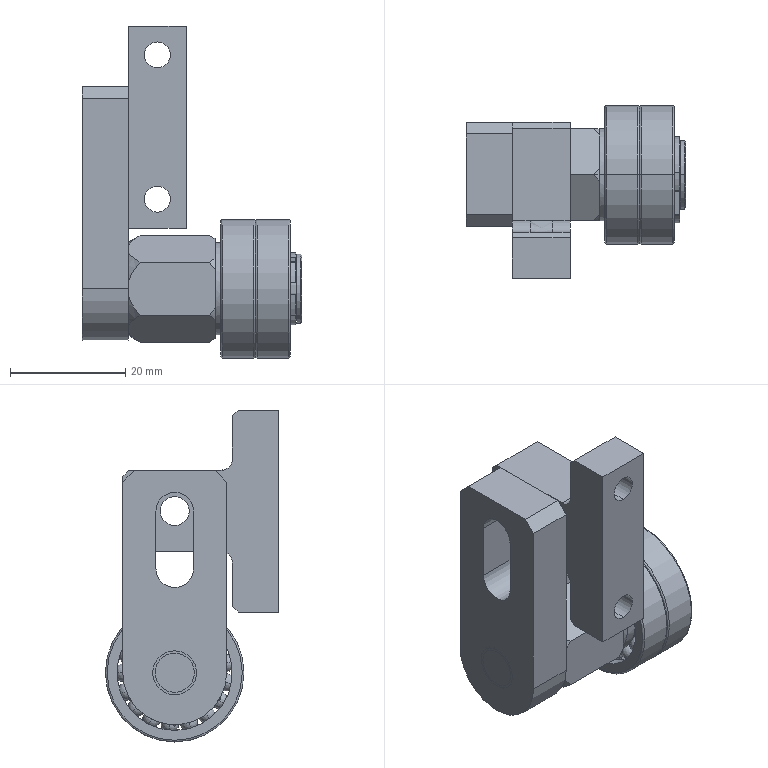Part | SolidWorks | features AEMSimFeature 1 | 6 solids | 343 faces | box 38 x 30 x 57.5 mm | volume 18168 mm3 | torus 124 | cylinder 71 | sphere 68 | plane 60 | cone 18 | spline 2 | commonest cylinder face diameters 16 x10 12 x8 20 x8 8 x6 1.5 x4 4 x4